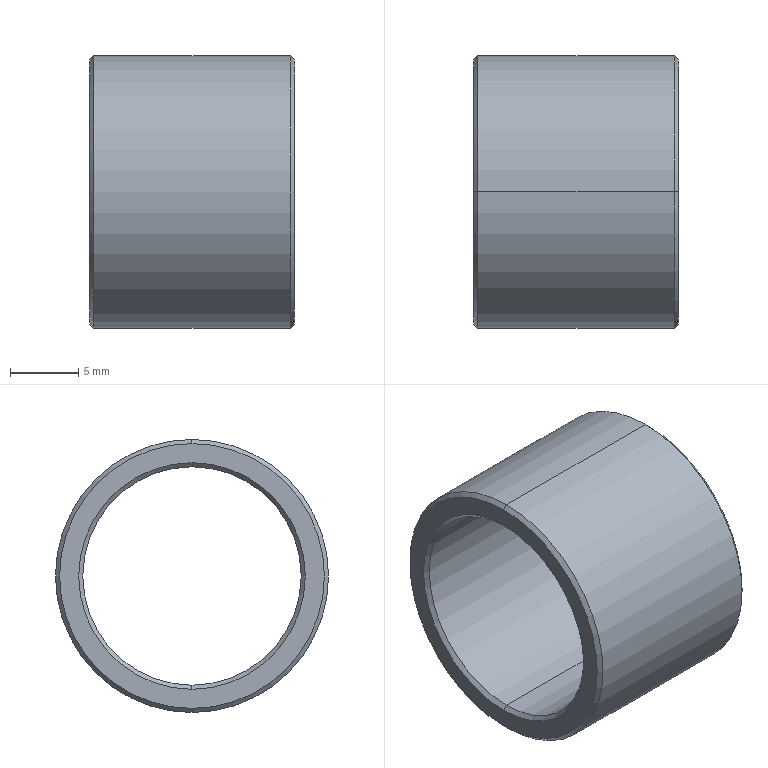Part | STEP file | 30B-162015T | 1 solid | 14 faces | box 15 x 20 x 20 mm | volume 1686 mm3 | cone 8 | cylinder 4 | plane 2 | commonest cylinder face diameters 16 x2 20 x2
STEP:
#1=CARTESIAN_POINT('',(0.,0.,-9.7));
#2=VERTEX_POINT('',#1);
#3=CARTESIAN_POINT('',(0.,0.,9.7));
#4=VERTEX_POINT('',#3);
#5=CARTESIAN_POINT('',(0.,0.,0.));
#6=DIRECTION('',(1.,0.,0.));
#7=DIRECTION('',(0.,0.,-1.));
#8=AXIS2_PLACEMENT_3D('',#5,#6,#7);
#9=CIRCLE('',#8,9.7);
#10=EDGE_CURVE('',#2,#4,#9,.T.);
#11=ORIENTED_EDGE('',*,*,#10,.T.);
#12=CARTESIAN_POINT('',(0.3,0.,10.));
#13=VERTEX_POINT('',#12);
#14=CARTESIAN_POINT('',(0.3,0.,10.));
#15=DIRECTION('',(0.7071,0.,0.7071));
#16=VECTOR('',#15,1000.);
#17=LINE('',#14,#16);
#18=EDGE_CURVE('',#4,#13,#17,.T.);
#19=ORIENTED_EDGE('',*,*,#18,.T.);
#20=CARTESIAN_POINT('',(0.3,0.,-10.));
#21=VERTEX_POINT('',#20);
#22=CARTESIAN_POINT('',(0.3,0.,0.));
#23=DIRECTION('',(1.,0.,0.));
#24=DIRECTION('',(0.,0.,-1.));
#25=AXIS2_PLACEMENT_3D('',#22,#23,#24);
#26=CIRCLE('',#25,10.);
#27=EDGE_CURVE('',#21,#13,#26,.T.);
#28=ORIENTED_EDGE('',*,*,#27,.F.);
#29=CARTESIAN_POINT('',(0.3,0.,-10.));
#30=DIRECTION('',(0.7071,0.,-0.7071));
#31=VECTOR('',#30,1000.);
#32=LINE('',#29,#31);
#33=EDGE_CURVE('',#2,#21,#32,.T.);
#34=ORIENTED_EDGE('',*,*,#33,.F.);
#35=EDGE_LOOP('',(#11,#19,#28,#34));
#36=FACE_OUTER_BOUND('',#35,.T.);
#37=CARTESIAN_POINT('',(0.3,0.,0.));
#38=DIRECTION('',(1.,0.,0.));
#39=DIRECTION('',(0.,0.,-1.));
#40=AXIS2_PLACEMENT_3D('',#37,#38,#39);
#41=CONICAL_SURFACE('',#40,10.,0.7854);
#42=ADVANCED_FACE('',(#36),#41,.T.);
#43=ORIENTED_EDGE('',*,*,#27,.T.);
#44=CARTESIAN_POINT('',(14.7,0.,10.));
#45=VERTEX_POINT('',#44);
#46=CARTESIAN_POINT('',(15.,0.,10.));
#47=DIRECTION('',(1.,0.,0.));
#48=VECTOR('',#47,1000.);
#49=LINE('',#46,#48);
#50=EDGE_CURVE('',#13,#45,#49,.T.);
#51=ORIENTED_EDGE('',*,*,#50,.T.);
#52=CARTESIAN_POINT('',(14.7,0.,-10.));
#53=VERTEX_POINT('',#52);
#54=CARTESIAN_POINT('',(14.7,0.,0.));
#55=DIRECTION('',(1.,0.,0.));
#56=DIRECTION('',(0.,0.,-1.));
#57=AXIS2_PLACEMENT_3D('',#54,#55,#56);
#58=CIRCLE('',#57,10.);
#59=EDGE_CURVE('',#53,#45,#58,.T.);
#60=ORIENTED_EDGE('',*,*,#59,.F.);
#61=CARTESIAN_POINT('',(15.,0.,-10.));
#62=DIRECTION('',(1.,0.,0.));
#63=VECTOR('',#62,1000.);
#64=LINE('',#61,#63);
#65=EDGE_CURVE('',#21,#53,#64,.T.);
#66=ORIENTED_EDGE('',*,*,#65,.F.);
#67=EDGE_LOOP('',(#43,#51,#60,#66));
#68=FACE_OUTER_BOUND('',#67,.T.);
#69=CARTESIAN_POINT('',(15.,0.,0.));
#70=DIRECTION('',(1.,0.,0.));
#71=DIRECTION('',(0.,0.,-1.));
#72=AXIS2_PLACEMENT_3D('',#69,#70,#71);
#73=CYLINDRICAL_SURFACE('',#72,10.);
#74=ADVANCED_FACE('',(#68),#73,.T.);
#75=CARTESIAN_POINT('',(15.,0.,-9.7));
#76=VERTEX_POINT('',#75);
#77=CARTESIAN_POINT('',(15.,0.,9.7));
#78=VERTEX_POINT('',#77);
#79=CARTESIAN_POINT('',(15.,0.,0.));
#80=DIRECTION('',(1.,0.,0.));
#81=DIRECTION('',(0.,0.,-1.));
#82=AXIS2_PLACEMENT_3D('',#79,#80,#81);
#83=CIRCLE('',#82,9.7);
#84=EDGE_CURVE('',#76,#78,#83,.T.);
#85=ORIENTED_EDGE('',*,*,#84,.F.);
#86=CARTESIAN_POINT('',(15.,0.,-9.7));
#87=DIRECTION('',(-0.7071,0.,-0.7071));
#88=VECTOR('',#87,1000.);
#89=LINE('',#86,#88);
#90=EDGE_CURVE('',#76,#53,#89,.T.);
#91=ORIENTED_EDGE('',*,*,#90,.T.);
#92=ORIENTED_EDGE('',*,*,#59,.T.);
#93=CARTESIAN_POINT('',(15.,0.,9.7));
#94=DIRECTION('',(-0.7071,0.,0.7071));
#95=VECTOR('',#94,1000.);
#96=LINE('',#93,#95);
#97=EDGE_CURVE('',#78,#45,#96,.T.);
#98=ORIENTED_EDGE('',*,*,#97,.F.);
#99=EDGE_LOOP('',(#85,#91,#92,#98));
#100=FACE_OUTER_BOUND('',#99,.T.);
#101=CARTESIAN_POINT('',(15.,0.,0.));
#102=DIRECTION('',(-1.,0.,0.));
#103=DIRECTION('',(0.,0.,1.));
#104=AXIS2_PLACEMENT_3D('',#101,#102,#103);
#105=CONICAL_SURFACE('',#104,9.7,0.7854);
#106=ADVANCED_FACE('',(#100),#105,.T.);
#107=CARTESIAN_POINT('',(14.7,0.,8.));
#108=VERTEX_POINT('',#107);
#109=CARTESIAN_POINT('',(14.7,0.,-8.));
#110=VERTEX_POINT('',#109);
#111=CARTESIAN_POINT('',(14.7,0.,0.));
#112=DIRECTION('',(1.,0.,0.));
#113=DIRECTION('',(0.,0.,-1.));
#114=AXIS2_PLACEMENT_3D('',#111,#112,#113);
#115=CIRCLE('',#114,8.);
#116=EDGE_CURVE('',#108,#110,#115,.T.);
#117=ORIENTED_EDGE('',*,*,#116,.F.);
#118=CARTESIAN_POINT('',(15.,0.,8.3));
#119=VERTEX_POINT('',#118);
#120=CARTESIAN_POINT('',(14.7,0.,8.));
#121=DIRECTION('',(0.7071,0.,0.7071));
#122=VECTOR('',#121,1000.);
#123=LINE('',#120,#122);
#124=EDGE_CURVE('',#108,#119,#123,.T.);
#125=ORIENTED_EDGE('',*,*,#124,.T.);
#126=CARTESIAN_POINT('',(15.,0.,-8.3));
#127=VERTEX_POINT('',#126);
#128=CARTESIAN_POINT('',(15.,0.,0.));
#129=DIRECTION('',(1.,0.,0.));
#130=DIRECTION('',(0.,0.,-1.));
#131=AXIS2_PLACEMENT_3D('',#128,#129,#130);
#132=CIRCLE('',#131,8.3);
#133=EDGE_CURVE('',#119,#127,#132,.T.);
#134=ORIENTED_EDGE('',*,*,#133,.T.);
#135=CARTESIAN_POINT('',(14.7,0.,-8.));
#136=DIRECTION('',(0.7071,0.,-0.7071));
#137=VECTOR('',#136,1000.);
#138=LINE('',#135,#137);
#139=EDGE_CURVE('',#110,#127,#138,.T.);
#140=ORIENTED_EDGE('',*,*,#139,.F.);
#141=EDGE_LOOP('',(#117,#125,#134,#140));
#142=FACE_OUTER_BOUND('',#141,.T.);
#143=CARTESIAN_POINT('',(14.7,0.,0.));
#144=DIRECTION('',(1.,0.,0.));
#145=DIRECTION('',(0.,0.,-1.));
#146=AXIS2_PLACEMENT_3D('',#143,#144,#145);
#147=CONICAL_SURFACE('',#146,8.,0.7854);
#148=ADVANCED_FACE('',(#142),#147,.F.);
#149=CARTESIAN_POINT('',(0.3,0.,8.));
#150=VERTEX_POINT('',#149);
#151=CARTESIAN_POINT('',(0.3,0.,-8.));
#152=VERTEX_POINT('',#151);
#153=CARTESIAN_POINT('',(0.3,0.,0.));
#154=DIRECTION('',(1.,0.,0.));
#155=DIRECTION('',(0.,0.,-1.));
#156=AXIS2_PLACEMENT_3D('',#153,#154,#155);
#157=CIRCLE('',#156,8.);
#158=EDGE_CURVE('',#150,#152,#157,.T.);
#159=ORIENTED_EDGE('',*,*,#158,.F.);
#160=CARTESIAN_POINT('',(15.,0.,8.));
#161=DIRECTION('',(1.,0.,0.));
#162=VECTOR('',#161,1000.);
#163=LINE('',#160,#162);
#164=EDGE_CURVE('',#150,#108,#163,.T.);
#165=ORIENTED_EDGE('',*,*,#164,.T.);
#166=ORIENTED_EDGE('',*,*,#116,.T.);
#167=CARTESIAN_POINT('',(15.,0.,-8.));
#168=DIRECTION('',(1.,0.,0.));
#169=VECTOR('',#168,1000.);
#170=LINE('',#167,#169);
#171=EDGE_CURVE('',#152,#110,#170,.T.);
#172=ORIENTED_EDGE('',*,*,#171,.F.);
#173=EDGE_LOOP('',(#159,#165,#166,#172));
#174=FACE_OUTER_BOUND('',#173,.T.);
#175=CARTESIAN_POINT('',(15.,0.,0.));
#176=DIRECTION('',(1.,0.,0.));
#177=DIRECTION('',(0.,0.,-1.));
#178=AXIS2_PLACEMENT_3D('',#175,#176,#177);
#179=CYLINDRICAL_SURFACE('',#178,8.);
#180=ADVANCED_FACE('',(#174),#179,.F.);
#181=ORIENTED_EDGE('',*,*,#158,.T.);
#182=CARTESIAN_POINT('',(0.,0.,-8.3));
#183=VERTEX_POINT('',#182);
#184=CARTESIAN_POINT('',(0.,0.,-8.3));
#185=DIRECTION('',(-0.7071,0.,-0.7071));
#186=VECTOR('',#185,1000.);
#187=LINE('',#184,#186);
#188=EDGE_CURVE('',#152,#183,#187,.T.);
#189=ORIENTED_EDGE('',*,*,#188,.T.);
#190=CARTESIAN_POINT('',(0.,0.,8.3));
#191=VERTEX_POINT('',#190);
#192=CARTESIAN_POINT('',(0.,0.,0.));
#193=DIRECTION('',(1.,0.,0.));
#194=DIRECTION('',(0.,0.,-1.));
#195=AXIS2_PLACEMENT_3D('',#192,#193,#194);
#196=CIRCLE('',#195,8.3);
#197=EDGE_CURVE('',#191,#183,#196,.T.);
#198=ORIENTED_EDGE('',*,*,#197,.F.);
#199=CARTESIAN_POINT('',(0.,0.,8.3));
#200=DIRECTION('',(-0.7071,0.,0.7071));
#201=VECTOR('',#200,1000.);
#202=LINE('',#199,#201);
#203=EDGE_CURVE('',#150,#191,#202,.T.);
#204=ORIENTED_EDGE('',*,*,#203,.F.);
#205=EDGE_LOOP('',(#181,#189,#198,#204));
#206=FACE_OUTER_BOUND('',#205,.T.);
#207=CARTESIAN_POINT('',(0.,0.,0.));
#208=DIRECTION('',(-1.,0.,0.));
#209=DIRECTION('',(0.,0.,1.));
#210=AXIS2_PLACEMENT_3D('',#207,#208,#209);
#211=CONICAL_SURFACE('',#210,8.3,0.7854);
#212=ADVANCED_FACE('',(#206),#211,.F.);
#213=ORIENTED_EDGE('',*,*,#197,.T.);
#214=CARTESIAN_POINT('',(0.,0.,0.));
#215=DIRECTION('',(1.,0.,0.));
#216=DIRECTION('',(0.,0.,-1.));
#217=AXIS2_PLACEMENT_3D('',#214,#215,#216);
#218=CIRCLE('',#217,8.3);
#219=EDGE_CURVE('',#183,#191,#218,.T.);
#220=ORIENTED_EDGE('',*,*,#219,.T.);
#221=EDGE_LOOP('',(#213,#220));
#222=FACE_BOUND('',#221,.T.);
#223=ORIENTED_EDGE('',*,*,#10,.F.);
#224=CARTESIAN_POINT('',(0.,0.,0.));
#225=DIRECTION('',(1.,0.,0.));
#226=DIRECTION('',(0.,0.,-1.));
#227=AXIS2_PLACEMENT_3D('',#224,#225,#226);
#228=CIRCLE('',#227,9.7);
#229=EDGE_CURVE('',#4,#2,#228,.T.);
#230=ORIENTED_EDGE('',*,*,#229,.F.);
#231=EDGE_LOOP('',(#223,#230));
#232=FACE_OUTER_BOUND('',#231,.T.);
#233=CARTESIAN_POINT('',(0.,9.7,0.));
#234=DIRECTION('',(-1.,0.,0.));
#235=DIRECTION('',(0.,0.,1.));
#236=AXIS2_PLACEMENT_3D('',#233,#234,#235);
#237=PLANE('',#236);
#238=ADVANCED_FACE('',(#222,#232),#237,.T.);
#239=ORIENTED_EDGE('',*,*,#188,.F.);
#240=CARTESIAN_POINT('',(0.3,0.,0.));
#241=DIRECTION('',(1.,0.,0.));
#242=DIRECTION('',(0.,0.,-1.));
#243=AXIS2_PLACEMENT_3D('',#240,#241,#242);
#244=CIRCLE('',#243,8.);
#245=EDGE_CURVE('',#152,#150,#244,.T.);
#246=ORIENTED_EDGE('',*,*,#245,.T.);
#247=ORIENTED_EDGE('',*,*,#203,.T.);
#248=ORIENTED_EDGE('',*,*,#219,.F.);
#249=EDGE_LOOP('',(#239,#246,#247,#248));
#250=FACE_OUTER_BOUND('',#249,.T.);
#251=CARTESIAN_POINT('',(0.,0.,0.));
#252=DIRECTION('',(-1.,0.,0.));
#253=DIRECTION('',(0.,0.,1.));
#254=AXIS2_PLACEMENT_3D('',#251,#252,#253);
#255=CONICAL_SURFACE('',#254,8.3,0.7854);
#256=ADVANCED_FACE('',(#250),#255,.F.);
#257=ORIENTED_EDGE('',*,*,#164,.F.);
#258=ORIENTED_EDGE('',*,*,#245,.F.);
#259=ORIENTED_EDGE('',*,*,#171,.T.);
#260=CARTESIAN_POINT('',(14.7,0.,0.));
#261=DIRECTION('',(1.,0.,0.));
#262=DIRECTION('',(0.,0.,-1.));
#263=AXIS2_PLACEMENT_3D('',#260,#261,#262);
#264=CIRCLE('',#263,8.);
#265=EDGE_CURVE('',#110,#108,#264,.T.);
#266=ORIENTED_EDGE('',*,*,#265,.T.);
#267=EDGE_LOOP('',(#257,#258,#259,#266));
#268=FACE_OUTER_BOUND('',#267,.T.);
#269=CARTESIAN_POINT('',(15.,0.,0.));
#270=DIRECTION('',(1.,0.,0.));
#271=DIRECTION('',(0.,0.,-1.));
#272=AXIS2_PLACEMENT_3D('',#269,#270,#271);
#273=CYLINDRICAL_SURFACE('',#272,8.);
#274=ADVANCED_FACE('',(#268),#273,.F.);
#275=ORIENTED_EDGE('',*,*,#124,.F.);
#276=ORIENTED_EDGE('',*,*,#265,.F.);
#277=ORIENTED_EDGE('',*,*,#139,.T.);
#278=CARTESIAN_POINT('',(15.,0.,0.));
#279=DIRECTION('',(1.,0.,0.));
#280=DIRECTION('',(0.,0.,-1.));
#281=AXIS2_PLACEMENT_3D('',#278,#279,#280);
#282=CIRCLE('',#281,8.3);
#283=EDGE_CURVE('',#127,#119,#282,.T.);
#284=ORIENTED_EDGE('',*,*,#283,.T.);
#285=EDGE_LOOP('',(#275,#276,#277,#284));
#286=FACE_OUTER_BOUND('',#285,.T.);
#287=CARTESIAN_POINT('',(14.7,0.,0.));
#288=DIRECTION('',(1.,0.,0.));
#289=DIRECTION('',(0.,0.,-1.));
#290=AXIS2_PLACEMENT_3D('',#287,#288,#289);
#291=CONICAL_SURFACE('',#290,8.,0.7854);
#292=ADVANCED_FACE('',(#286),#291,.F.);
#293=CARTESIAN_POINT('',(15.,0.,0.));
#294=DIRECTION('',(1.,0.,0.));
#295=DIRECTION('',(0.,0.,-1.));
#296=AXIS2_PLACEMENT_3D('',#293,#294,#295);
#297=CIRCLE('',#296,9.7);
#298=EDGE_CURVE('',#78,#76,#297,.T.);
#299=ORIENTED_EDGE('',*,*,#298,.T.);
#300=ORIENTED_EDGE('',*,*,#84,.T.);
#301=EDGE_LOOP('',(#299,#300));
#302=FACE_OUTER_BOUND('',#301,.T.);
#303=ORIENTED_EDGE('',*,*,#283,.F.);
#304=ORIENTED_EDGE('',*,*,#133,.F.);
#305=EDGE_LOOP('',(#303,#304));
#306=FACE_BOUND('',#305,.T.);
#307=CARTESIAN_POINT('',(15.,8.3,0.));
#308=DIRECTION('',(1.,0.,0.));
#309=DIRECTION('',(0.,0.,-1.));
#310=AXIS2_PLACEMENT_3D('',#307,#308,#309);
#311=PLANE('',#310);
#312=ADVANCED_FACE('',(#302,#306),#311,.T.);
#313=ORIENTED_EDGE('',*,*,#90,.F.);
#314=ORIENTED_EDGE('',*,*,#298,.F.);
#315=ORIENTED_EDGE('',*,*,#97,.T.);
#316=CARTESIAN_POINT('',(14.7,0.,0.));
#317=DIRECTION('',(1.,0.,0.));
#318=DIRECTION('',(0.,0.,-1.));
#319=AXIS2_PLACEMENT_3D('',#316,#317,#318);
#320=CIRCLE('',#319,10.);
#321=EDGE_CURVE('',#45,#53,#320,.T.);
#322=ORIENTED_EDGE('',*,*,#321,.T.);
#323=EDGE_LOOP('',(#313,#314,#315,#322));
#324=FACE_OUTER_BOUND('',#323,.T.);
#325=CARTESIAN_POINT('',(15.,0.,0.));
#326=DIRECTION('',(-1.,0.,0.));
#327=DIRECTION('',(0.,0.,1.));
#328=AXIS2_PLACEMENT_3D('',#325,#326,#327);
#329=CONICAL_SURFACE('',#328,9.7,0.7854);
#330=ADVANCED_FACE('',(#324),#329,.T.);
#331=ORIENTED_EDGE('',*,*,#50,.F.);
#332=CARTESIAN_POINT('',(0.3,0.,0.));
#333=DIRECTION('',(1.,0.,0.));
#334=DIRECTION('',(0.,0.,-1.));
#335=AXIS2_PLACEMENT_3D('',#332,#333,#334);
#336=CIRCLE('',#335,10.);
#337=EDGE_CURVE('',#13,#21,#336,.T.);
#338=ORIENTED_EDGE('',*,*,#337,.T.);
#339=ORIENTED_EDGE('',*,*,#65,.T.);
#340=ORIENTED_EDGE('',*,*,#321,.F.);
#341=EDGE_LOOP('',(#331,#338,#339,#340));
#342=FACE_OUTER_BOUND('',#341,.T.);
#343=CARTESIAN_POINT('',(15.,0.,0.));
#344=DIRECTION('',(1.,0.,0.));
#345=DIRECTION('',(0.,0.,-1.));
#346=AXIS2_PLACEMENT_3D('',#343,#344,#345);
#347=CYLINDRICAL_SURFACE('',#346,10.);
#348=ADVANCED_FACE('',(#342),#347,.T.);
#349=ORIENTED_EDGE('',*,*,#18,.F.);
#350=ORIENTED_EDGE('',*,*,#229,.T.);
#351=ORIENTED_EDGE('',*,*,#33,.T.);
#352=ORIENTED_EDGE('',*,*,#337,.F.);
#353=EDGE_LOOP('',(#349,#350,#351,#352));
#354=FACE_OUTER_BOUND('',#353,.T.);
#355=CARTESIAN_POINT('',(0.3,0.,0.));
#356=DIRECTION('',(1.,0.,0.));
#357=DIRECTION('',(0.,0.,-1.));
#358=AXIS2_PLACEMENT_3D('',#355,#356,#357);
#359=CONICAL_SURFACE('',#358,10.,0.7854);
#360=ADVANCED_FACE('',(#354),#359,.T.);
#361=CLOSED_SHELL('',(#42,#74,#106,#148,#180,#212,#238,#256,#274,#292,#312,#330,#348,#360));
#362=MANIFOLD_SOLID_BREP('',#361);
#363=CARTESIAN_POINT('',(0.,0.,0.));
#364=DIRECTION('',(0.,0.,1.));
#365=DIRECTION('',(1.,0.,0.));
#366=AXIS2_PLACEMENT_3D('',#363,#364,#365);
#367=(LENGTH_UNIT()NAMED_UNIT(*)SI_UNIT(.MILLI.,.METRE.));
#368=UNCERTAINTY_MEASURE_WITH_UNIT(LENGTH_MEASURE(0.00001),#367,'','');
#369=(NAMED_UNIT(*)PLANE_ANGLE_UNIT()SI_UNIT($,.RADIAN.));
#370=(NAMED_UNIT(*)SI_UNIT($,.STERADIAN.)SOLID_ANGLE_UNIT());
#371=(GEOMETRIC_REPRESENTATION_CONTEXT(3)GLOBAL_UNCERTAINTY_ASSIGNED_CONTEXT((#368))GLOBAL_UNIT_ASSIGNED_CONTEXT((#367,#369,#370))REPRESENTATION_CONTEXT('',''));
#372=ADVANCED_BREP_SHAPE_REPRESENTATION('',(#362,#366),#371);